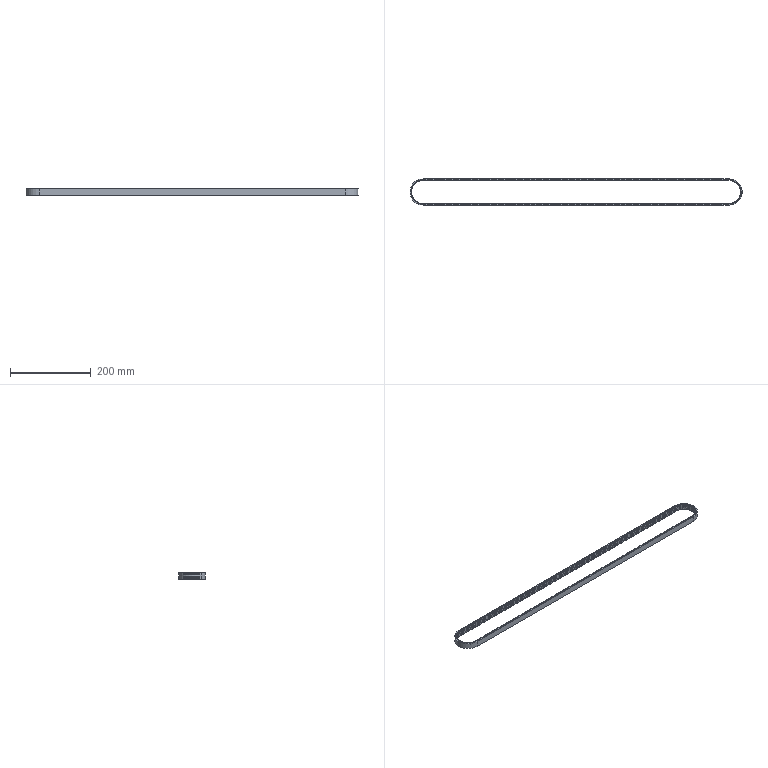Part | SolidWorks | features CurvePattern 3, ICE 3, Extrusion 1 | 1 solid | 828 faces | box 825 x 65 x 15 mm | volume 85490 mm3 | cylinder 470 | plane 358 | commonest cylinder face diameters 3 x421 60 x46 65 x3